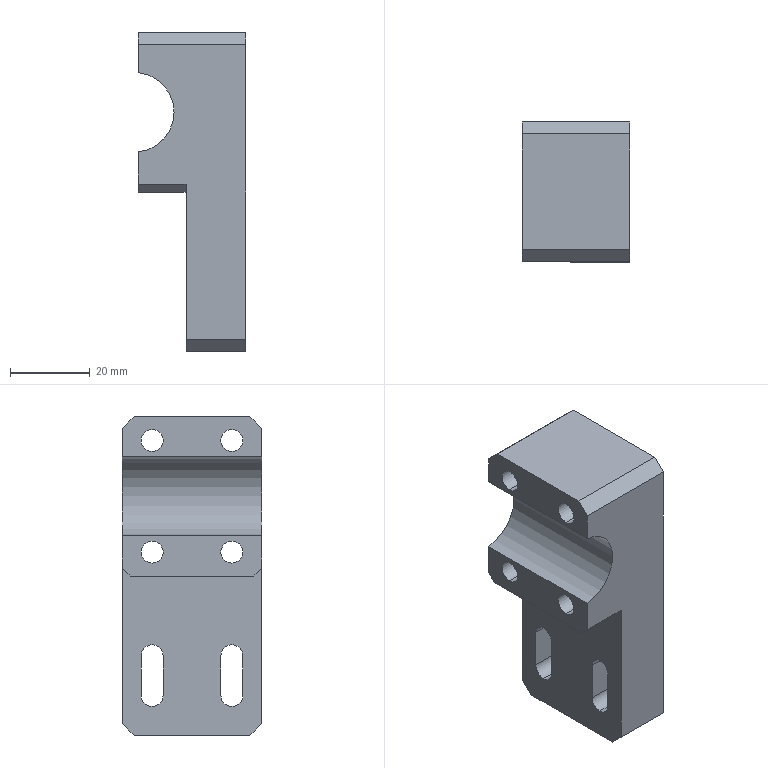Part | SolidWorks | features Chamfer 2, HoleWzd 2, Extrusion 1, ICE 1 | 1 solid | 58 faces | box 27 x 35 x 80 mm | volume 44069 mm3 | cylinder 29 | plane 29 | commonest cylinder face diameters 5.5 x14 10 x14 20 x1